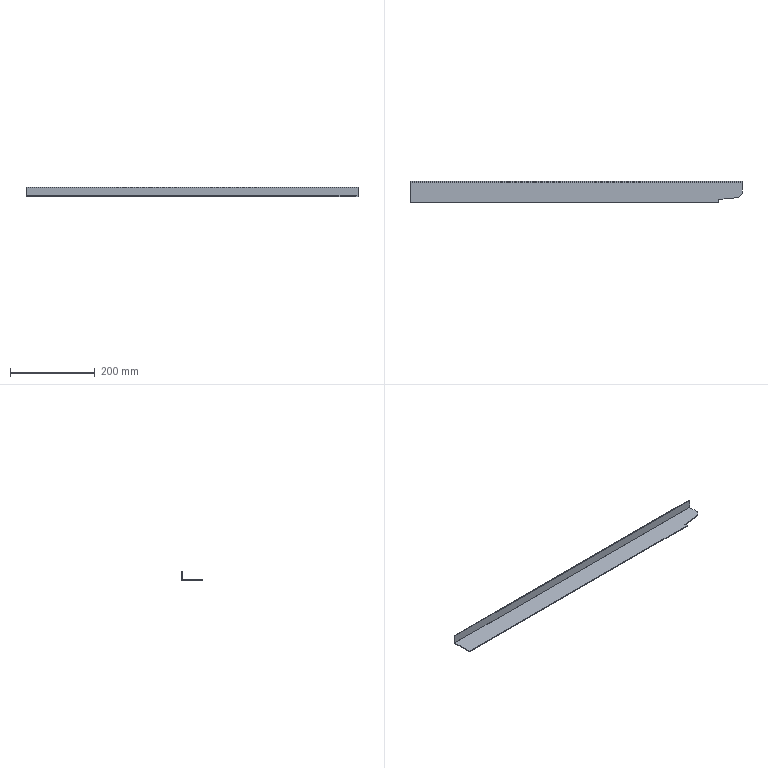Part | SolidWorks | 1 solid | 18 faces | box 783.5 x 50 x 22 mm | volume 107737 mm3 | plane 16 | cylinder 2 | commonest cylinder face diameters 0.2 x1 4.2 x1
STEP:
#1=CARTESIAN_POINT('',(335.25,-25.,-2.));
#2=VERTEX_POINT('',#1);
#3=CARTESIAN_POINT('',(335.25,-17.499,-2.));
#4=VERTEX_POINT('',#3);
#5=CARTESIAN_POINT('',(335.25,0.,-2.));
#6=DIRECTION('',(0.,1.,0.));
#7=VECTOR('',#6,1000.);
#8=LINE('',#5,#7);
#9=EDGE_CURVE('',#2,#4,#8,.T.);
#10=ORIENTED_EDGE('',*,*,#9,.F.);
#11=CARTESIAN_POINT('',(-391.75,-25.,-2.));
#12=VERTEX_POINT('',#11);
#13=CARTESIAN_POINT('',(391.75,-25.,-2.));
#14=DIRECTION('',(1.,0.,0.));
#15=VECTOR('',#14,1000.);
#16=LINE('',#13,#15);
#17=EDGE_CURVE('',#12,#2,#16,.T.);
#18=ORIENTED_EDGE('',*,*,#17,.F.);
#19=CARTESIAN_POINT('',(-391.75,22.9,-2.));
#20=VERTEX_POINT('',#19);
#21=CARTESIAN_POINT('',(-391.75,-25.,-2.));
#22=DIRECTION('',(0.,-1.,0.));
#23=VECTOR('',#22,1000.);
#24=LINE('',#21,#23);
#25=EDGE_CURVE('',#20,#12,#24,.T.);
#26=ORIENTED_EDGE('',*,*,#25,.F.);
#27=CARTESIAN_POINT('',(391.75,22.9,-2.));
#28=VERTEX_POINT('',#27);
#29=CARTESIAN_POINT('',(-391.75,22.9,-2.));
#30=DIRECTION('',(1.,0.,0.));
#31=VECTOR('',#30,1000.);
#32=LINE('',#29,#31);
#33=EDGE_CURVE('',#20,#28,#32,.T.);
#34=ORIENTED_EDGE('',*,*,#33,.T.);
#35=CARTESIAN_POINT('',(391.75,-3.027,-2.));
#36=VERTEX_POINT('',#35);
#37=CARTESIAN_POINT('',(391.75,-25.,-2.));
#38=DIRECTION('',(0.,1.,0.));
#39=VECTOR('',#38,1000.);
#40=LINE('',#37,#39);
#41=EDGE_CURVE('',#36,#28,#40,.T.);
#42=ORIENTED_EDGE('',*,*,#41,.F.);
#43=CARTESIAN_POINT('',(382.795,-12.972,-2.));
#44=VERTEX_POINT('',#43);
#45=CARTESIAN_POINT('',(382.795,-12.972,-2.));
#46=DIRECTION('',(0.6691,0.7431,0.));
#47=VECTOR('',#46,1000.);
#48=LINE('',#45,#47);
#49=EDGE_CURVE('',#44,#36,#48,.T.);
#50=ORIENTED_EDGE('',*,*,#49,.F.);
#51=CARTESIAN_POINT('',(339.727,-17.499,-2.));
#52=VERTEX_POINT('',#51);
#53=CARTESIAN_POINT('',(339.727,-17.499,-2.));
#54=DIRECTION('',(0.9945,0.1045,0.));
#55=VECTOR('',#54,1000.);
#56=LINE('',#53,#55);
#57=EDGE_CURVE('',#52,#44,#56,.T.);
#58=ORIENTED_EDGE('',*,*,#57,.F.);
#59=CARTESIAN_POINT('',(0.,-17.499,-2.));
#60=DIRECTION('',(1.,0.,0.));
#61=VECTOR('',#60,1000.);
#62=LINE('',#59,#61);
#63=EDGE_CURVE('',#4,#52,#62,.T.);
#64=ORIENTED_EDGE('',*,*,#63,.F.);
#65=EDGE_LOOP('',(#10,#18,#26,#34,#42,#50,#58,#64));
#66=FACE_OUTER_BOUND('',#65,.T.);
#67=CARTESIAN_POINT('',(0.,0.,-2.));
#68=DIRECTION('',(0.,0.,1.));
#69=DIRECTION('',(1.,0.,0.));
#70=AXIS2_PLACEMENT_3D('',#67,#68,#69);
#71=PLANE('',#70);
#72=ADVANCED_FACE('',(#66),#71,.F.);
#73=CARTESIAN_POINT('',(-391.75,-25.,0.));
#74=VERTEX_POINT('',#73);
#75=CARTESIAN_POINT('',(335.25,-25.,0.));
#76=VERTEX_POINT('',#75);
#77=CARTESIAN_POINT('',(391.75,-25.,0.));
#78=DIRECTION('',(1.,0.,0.));
#79=VECTOR('',#78,1000.);
#80=LINE('',#77,#79);
#81=EDGE_CURVE('',#74,#76,#80,.T.);
#82=ORIENTED_EDGE('',*,*,#81,.T.);
#83=CARTESIAN_POINT('',(335.25,-17.499,0.));
#84=VERTEX_POINT('',#83);
#85=CARTESIAN_POINT('',(335.25,-25.,0.));
#86=DIRECTION('',(0.,1.,0.));
#87=VECTOR('',#86,1000.);
#88=LINE('',#85,#87);
#89=EDGE_CURVE('',#76,#84,#88,.T.);
#90=ORIENTED_EDGE('',*,*,#89,.T.);
#91=CARTESIAN_POINT('',(339.727,-17.499,0.));
#92=VERTEX_POINT('',#91);
#93=CARTESIAN_POINT('',(335.25,-17.499,0.));
#94=DIRECTION('',(1.,0.,0.));
#95=VECTOR('',#94,1000.);
#96=LINE('',#93,#95);
#97=EDGE_CURVE('',#84,#92,#96,.T.);
#98=ORIENTED_EDGE('',*,*,#97,.T.);
#99=CARTESIAN_POINT('',(382.795,-12.972,0.));
#100=VERTEX_POINT('',#99);
#101=CARTESIAN_POINT('',(339.727,-17.499,0.));
#102=DIRECTION('',(0.9945,0.1045,0.));
#103=VECTOR('',#102,1000.);
#104=LINE('',#101,#103);
#105=EDGE_CURVE('',#92,#100,#104,.T.);
#106=ORIENTED_EDGE('',*,*,#105,.T.);
#107=CARTESIAN_POINT('',(391.75,-3.027,0.));
#108=VERTEX_POINT('',#107);
#109=CARTESIAN_POINT('',(382.795,-12.972,0.));
#110=DIRECTION('',(0.6691,0.7431,0.));
#111=VECTOR('',#110,1000.);
#112=LINE('',#109,#111);
#113=EDGE_CURVE('',#100,#108,#112,.T.);
#114=ORIENTED_EDGE('',*,*,#113,.T.);
#115=CARTESIAN_POINT('',(391.75,22.9,0.));
#116=VERTEX_POINT('',#115);
#117=CARTESIAN_POINT('',(391.75,-25.,0.));
#118=DIRECTION('',(0.,1.,0.));
#119=VECTOR('',#118,1000.);
#120=LINE('',#117,#119);
#121=EDGE_CURVE('',#108,#116,#120,.T.);
#122=ORIENTED_EDGE('',*,*,#121,.T.);
#123=CARTESIAN_POINT('',(-391.75,22.9,0.));
#124=VERTEX_POINT('',#123);
#125=CARTESIAN_POINT('',(-391.75,22.9,0.));
#126=DIRECTION('',(1.,0.,0.));
#127=VECTOR('',#126,1000.);
#128=LINE('',#125,#127);
#129=EDGE_CURVE('',#124,#116,#128,.T.);
#130=ORIENTED_EDGE('',*,*,#129,.F.);
#131=CARTESIAN_POINT('',(-391.75,-25.,0.));
#132=DIRECTION('',(0.,-1.,0.));
#133=VECTOR('',#132,1000.);
#134=LINE('',#131,#133);
#135=EDGE_CURVE('',#124,#74,#134,.T.);
#136=ORIENTED_EDGE('',*,*,#135,.T.);
#137=EDGE_LOOP('',(#82,#90,#98,#106,#114,#122,#130,#136));
#138=FACE_OUTER_BOUND('',#137,.T.);
#139=CARTESIAN_POINT('',(0.,0.,0.));
#140=DIRECTION('',(0.,0.,1.));
#141=DIRECTION('',(1.,0.,0.));
#142=AXIS2_PLACEMENT_3D('',#139,#140,#141);
#143=PLANE('',#142);
#144=ADVANCED_FACE('',(#138),#143,.T.);
#145=ORIENTED_EDGE('',*,*,#121,.F.);
#146=CARTESIAN_POINT('',(391.75,-3.027,0.));
#147=DIRECTION('',(0.,0.,-1.));
#148=VECTOR('',#147,1000.);
#149=LINE('',#146,#148);
#150=EDGE_CURVE('',#108,#36,#149,.T.);
#151=ORIENTED_EDGE('',*,*,#150,.T.);
#152=ORIENTED_EDGE('',*,*,#41,.T.);
#153=CARTESIAN_POINT('',(391.75,22.9,0.));
#154=DIRECTION('',(0.,0.,-1.));
#155=VECTOR('',#154,1000.);
#156=LINE('',#153,#155);
#157=EDGE_CURVE('',#116,#28,#156,.T.);
#158=ORIENTED_EDGE('',*,*,#157,.F.);
#159=EDGE_LOOP('',(#145,#151,#152,#158));
#160=FACE_OUTER_BOUND('',#159,.T.);
#161=CARTESIAN_POINT('',(391.75,-25.,-2.));
#162=DIRECTION('',(1.,0.,0.));
#163=DIRECTION('',(0.,0.,-1.));
#164=AXIS2_PLACEMENT_3D('',#161,#162,#163);
#165=PLANE('',#164);
#166=ADVANCED_FACE('',(#160),#165,.T.);
#167=ORIENTED_EDGE('',*,*,#17,.T.);
#168=CARTESIAN_POINT('',(335.25,-25.,0.));
#169=DIRECTION('',(0.,0.,-1.));
#170=VECTOR('',#169,1000.);
#171=LINE('',#168,#170);
#172=EDGE_CURVE('',#76,#2,#171,.T.);
#173=ORIENTED_EDGE('',*,*,#172,.F.);
#174=ORIENTED_EDGE('',*,*,#81,.F.);
#175=CARTESIAN_POINT('',(-391.75,-25.,-2.));
#176=DIRECTION('',(0.,0.,1.));
#177=VECTOR('',#176,1000.);
#178=LINE('',#175,#177);
#179=EDGE_CURVE('',#12,#74,#178,.T.);
#180=ORIENTED_EDGE('',*,*,#179,.F.);
#181=EDGE_LOOP('',(#167,#173,#174,#180));
#182=FACE_OUTER_BOUND('',#181,.T.);
#183=CARTESIAN_POINT('',(391.75,-25.,-2.));
#184=DIRECTION('',(0.,-1.,0.));
#185=DIRECTION('',(1.,0.,0.));
#186=AXIS2_PLACEMENT_3D('',#183,#184,#185);
#187=PLANE('',#186);
#188=ADVANCED_FACE('',(#182),#187,.T.);
#189=ORIENTED_EDGE('',*,*,#135,.F.);
#190=CARTESIAN_POINT('',(-391.75,22.9,0.));
#191=DIRECTION('',(0.,0.,-1.));
#192=VECTOR('',#191,1000.);
#193=LINE('',#190,#192);
#194=EDGE_CURVE('',#124,#20,#193,.T.);
#195=ORIENTED_EDGE('',*,*,#194,.T.);
#196=ORIENTED_EDGE('',*,*,#25,.T.);
#197=ORIENTED_EDGE('',*,*,#179,.T.);
#198=EDGE_LOOP('',(#189,#195,#196,#197));
#199=FACE_OUTER_BOUND('',#198,.T.);
#200=CARTESIAN_POINT('',(-391.75,-25.,-2.));
#201=DIRECTION('',(-1.,0.,0.));
#202=DIRECTION('',(0.,0.,1.));
#203=AXIS2_PLACEMENT_3D('',#200,#201,#202);
#204=PLANE('',#203);
#205=ADVANCED_FACE('',(#199),#204,.T.);
#206=CARTESIAN_POINT('',(391.75,23.,0.1));
#207=VERTEX_POINT('',#206);
#208=CARTESIAN_POINT('',(391.75,25.,0.1));
#209=VERTEX_POINT('',#208);
#210=CARTESIAN_POINT('',(391.75,25.,0.1));
#211=DIRECTION('',(0.,1.,0.));
#212=VECTOR('',#211,1000.);
#213=LINE('',#210,#212);
#214=EDGE_CURVE('',#207,#209,#213,.T.);
#215=ORIENTED_EDGE('',*,*,#214,.F.);
#216=CARTESIAN_POINT('',(391.75,22.9,0.1));
#217=DIRECTION('',(1.,0.,0.));
#218=DIRECTION('',(0.,0.,1.));
#219=AXIS2_PLACEMENT_3D('',#216,#217,#218);
#220=CIRCLE('',#219,0.1);
#221=EDGE_CURVE('',#116,#207,#220,.T.);
#222=ORIENTED_EDGE('',*,*,#221,.F.);
#223=ORIENTED_EDGE('',*,*,#157,.T.);
#224=CARTESIAN_POINT('',(391.75,22.9,0.1));
#225=DIRECTION('',(1.,0.,0.));
#226=DIRECTION('',(0.,0.,1.));
#227=AXIS2_PLACEMENT_3D('',#224,#225,#226);
#228=CIRCLE('',#227,2.1);
#229=EDGE_CURVE('',#28,#209,#228,.T.);
#230=ORIENTED_EDGE('',*,*,#229,.T.);
#231=EDGE_LOOP('',(#215,#222,#223,#230));
#232=FACE_OUTER_BOUND('',#231,.T.);
#233=CARTESIAN_POINT('',(391.75,22.9,0.1));
#234=DIRECTION('',(1.,0.,0.));
#235=DIRECTION('',(0.,0.,-1.));
#236=AXIS2_PLACEMENT_3D('',#233,#234,#235);
#237=PLANE('',#236);
#238=ADVANCED_FACE('',(#232),#237,.T.);
#239=CARTESIAN_POINT('',(-391.75,23.,0.1));
#240=VERTEX_POINT('',#239);
#241=CARTESIAN_POINT('',(-391.75,22.9,0.1));
#242=DIRECTION('',(-1.,0.,0.));
#243=DIRECTION('',(0.,0.,1.));
#244=AXIS2_PLACEMENT_3D('',#241,#242,#243);
#245=CIRCLE('',#244,0.1);
#246=EDGE_CURVE('',#240,#124,#245,.T.);
#247=ORIENTED_EDGE('',*,*,#246,.F.);
#248=CARTESIAN_POINT('',(-391.75,25.,0.1));
#249=VERTEX_POINT('',#248);
#250=CARTESIAN_POINT('',(-391.75,23.,0.1));
#251=DIRECTION('',(0.,1.,0.));
#252=VECTOR('',#251,1000.);
#253=LINE('',#250,#252);
#254=EDGE_CURVE('',#240,#249,#253,.T.);
#255=ORIENTED_EDGE('',*,*,#254,.T.);
#256=CARTESIAN_POINT('',(-391.75,22.9,0.1));
#257=DIRECTION('',(-1.,0.,0.));
#258=DIRECTION('',(0.,0.,1.));
#259=AXIS2_PLACEMENT_3D('',#256,#257,#258);
#260=CIRCLE('',#259,2.1);
#261=EDGE_CURVE('',#249,#20,#260,.T.);
#262=ORIENTED_EDGE('',*,*,#261,.T.);
#263=ORIENTED_EDGE('',*,*,#194,.F.);
#264=EDGE_LOOP('',(#247,#255,#262,#263));
#265=FACE_OUTER_BOUND('',#264,.T.);
#266=CARTESIAN_POINT('',(-391.75,22.9,0.1));
#267=DIRECTION('',(1.,0.,0.));
#268=DIRECTION('',(0.,0.,-1.));
#269=AXIS2_PLACEMENT_3D('',#266,#267,#268);
#270=PLANE('',#269);
#271=ADVANCED_FACE('',(#265),#270,.F.);
#272=ORIENTED_EDGE('',*,*,#33,.F.);
#273=ORIENTED_EDGE('',*,*,#261,.F.);
#274=CARTESIAN_POINT('',(0.,25.,0.1));
#275=DIRECTION('',(-1.,0.,0.));
#276=VECTOR('',#275,1000.);
#277=LINE('',#274,#276);
#278=EDGE_CURVE('',#209,#249,#277,.T.);
#279=ORIENTED_EDGE('',*,*,#278,.F.);
#280=ORIENTED_EDGE('',*,*,#229,.F.);
#281=EDGE_LOOP('',(#272,#273,#279,#280));
#282=FACE_OUTER_BOUND('',#281,.T.);
#283=CARTESIAN_POINT('',(-391.75,22.9,0.1));
#284=DIRECTION('',(-1.,0.,0.));
#285=DIRECTION('',(0.,1.,0.));
#286=AXIS2_PLACEMENT_3D('',#283,#284,#285);
#287=CYLINDRICAL_SURFACE('',#286,2.1);
#288=ADVANCED_FACE('',(#282),#287,.T.);
#289=ORIENTED_EDGE('',*,*,#129,.T.);
#290=ORIENTED_EDGE('',*,*,#221,.T.);
#291=CARTESIAN_POINT('',(391.75,23.,0.1));
#292=DIRECTION('',(-1.,0.,0.));
#293=VECTOR('',#292,1000.);
#294=LINE('',#291,#293);
#295=EDGE_CURVE('',#207,#240,#294,.T.);
#296=ORIENTED_EDGE('',*,*,#295,.T.);
#297=ORIENTED_EDGE('',*,*,#246,.T.);
#298=EDGE_LOOP('',(#289,#290,#296,#297));
#299=FACE_OUTER_BOUND('',#298,.T.);
#300=CARTESIAN_POINT('',(-391.75,22.9,0.1));
#301=DIRECTION('',(-1.,0.,0.));
#302=DIRECTION('',(0.,1.,0.));
#303=AXIS2_PLACEMENT_3D('',#300,#301,#302);
#304=CYLINDRICAL_SURFACE('',#303,0.1);
#305=ADVANCED_FACE('',(#299),#304,.F.);
#306=CARTESIAN_POINT('',(-391.75,25.,20.));
#307=VERTEX_POINT('',#306);
#308=CARTESIAN_POINT('',(-391.75,25.,0.));
#309=DIRECTION('',(0.,0.,-1.));
#310=VECTOR('',#309,1000.);
#311=LINE('',#308,#310);
#312=EDGE_CURVE('',#307,#249,#311,.T.);
#313=ORIENTED_EDGE('',*,*,#312,.T.);
#314=ORIENTED_EDGE('',*,*,#254,.F.);
#315=CARTESIAN_POINT('',(-391.75,23.,20.));
#316=VERTEX_POINT('',#315);
#317=CARTESIAN_POINT('',(-391.75,23.,0.));
#318=DIRECTION('',(0.,0.,-1.));
#319=VECTOR('',#318,1000.);
#320=LINE('',#317,#319);
#321=EDGE_CURVE('',#316,#240,#320,.T.);
#322=ORIENTED_EDGE('',*,*,#321,.F.);
#323=CARTESIAN_POINT('',(-391.75,25.,20.));
#324=DIRECTION('',(0.,-1.,0.));
#325=VECTOR('',#324,1000.);
#326=LINE('',#323,#325);
#327=EDGE_CURVE('',#307,#316,#326,.T.);
#328=ORIENTED_EDGE('',*,*,#327,.F.);
#329=EDGE_LOOP('',(#313,#314,#322,#328));
#330=FACE_OUTER_BOUND('',#329,.T.);
#331=CARTESIAN_POINT('',(-391.75,25.,0.));
#332=DIRECTION('',(-1.,0.,0.));
#333=DIRECTION('',(0.,-1.,0.));
#334=AXIS2_PLACEMENT_3D('',#331,#332,#333);
#335=PLANE('',#334);
#336=ADVANCED_FACE('',(#330),#335,.T.);
#337=CARTESIAN_POINT('',(391.75,23.,20.));
#338=VERTEX_POINT('',#337);
#339=CARTESIAN_POINT('',(391.75,23.,0.));
#340=DIRECTION('',(0.,0.,1.));
#341=VECTOR('',#340,1000.);
#342=LINE('',#339,#341);
#343=EDGE_CURVE('',#207,#338,#342,.T.);
#344=ORIENTED_EDGE('',*,*,#343,.F.);
#345=ORIENTED_EDGE('',*,*,#214,.T.);
#346=CARTESIAN_POINT('',(391.75,25.,20.));
#347=VERTEX_POINT('',#346);
#348=CARTESIAN_POINT('',(391.75,25.,20.));
#349=DIRECTION('',(0.,0.,1.));
#350=VECTOR('',#349,1000.);
#351=LINE('',#348,#350);
#352=EDGE_CURVE('',#209,#347,#351,.T.);
#353=ORIENTED_EDGE('',*,*,#352,.T.);
#354=CARTESIAN_POINT('',(391.75,25.,20.));
#355=DIRECTION('',(0.,-1.,0.));
#356=VECTOR('',#355,1000.);
#357=LINE('',#354,#356);
#358=EDGE_CURVE('',#347,#338,#357,.T.);
#359=ORIENTED_EDGE('',*,*,#358,.T.);
#360=EDGE_LOOP('',(#344,#345,#353,#359));
#361=FACE_OUTER_BOUND('',#360,.T.);
#362=CARTESIAN_POINT('',(391.75,25.,20.));
#363=DIRECTION('',(1.,0.,0.));
#364=DIRECTION('',(0.,1.,0.));
#365=AXIS2_PLACEMENT_3D('',#362,#363,#364);
#366=PLANE('',#365);
#367=ADVANCED_FACE('',(#361),#366,.T.);
#368=ORIENTED_EDGE('',*,*,#352,.F.);
#369=ORIENTED_EDGE('',*,*,#278,.T.);
#370=ORIENTED_EDGE('',*,*,#312,.F.);
#371=CARTESIAN_POINT('',(-391.75,25.,20.));
#372=DIRECTION('',(-1.,0.,0.));
#373=VECTOR('',#372,1000.);
#374=LINE('',#371,#373);
#375=EDGE_CURVE('',#347,#307,#374,.T.);
#376=ORIENTED_EDGE('',*,*,#375,.F.);
#377=EDGE_LOOP('',(#368,#369,#370,#376));
#378=FACE_OUTER_BOUND('',#377,.T.);
#379=CARTESIAN_POINT('',(0.,25.,0.));
#380=DIRECTION('',(0.,1.,0.));
#381=DIRECTION('',(0.,0.,1.));
#382=AXIS2_PLACEMENT_3D('',#379,#380,#381);
#383=PLANE('',#382);
#384=ADVANCED_FACE('',(#378),#383,.T.);
#385=ORIENTED_EDGE('',*,*,#295,.F.);
#386=ORIENTED_EDGE('',*,*,#343,.T.);
#387=CARTESIAN_POINT('',(0.,23.,20.));
#388=DIRECTION('',(-1.,0.,0.));
#389=VECTOR('',#388,1000.);
#390=LINE('',#387,#389);
#391=EDGE_CURVE('',#338,#316,#390,.T.);
#392=ORIENTED_EDGE('',*,*,#391,.T.);
#393=ORIENTED_EDGE('',*,*,#321,.T.);
#394=EDGE_LOOP('',(#385,#386,#392,#393));
#395=FACE_OUTER_BOUND('',#394,.T.);
#396=CARTESIAN_POINT('',(0.,23.,0.));
#397=DIRECTION('',(0.,1.,0.));
#398=DIRECTION('',(0.,0.,1.));
#399=AXIS2_PLACEMENT_3D('',#396,#397,#398);
#400=PLANE('',#399);
#401=ADVANCED_FACE('',(#395),#400,.F.);
#402=ORIENTED_EDGE('',*,*,#391,.F.);
#403=ORIENTED_EDGE('',*,*,#358,.F.);
#404=ORIENTED_EDGE('',*,*,#375,.T.);
#405=ORIENTED_EDGE('',*,*,#327,.T.);
#406=EDGE_LOOP('',(#402,#403,#404,#405));
#407=FACE_OUTER_BOUND('',#406,.T.);
#408=CARTESIAN_POINT('',(-391.75,25.,20.));
#409=DIRECTION('',(0.,0.,1.));
#410=DIRECTION('',(0.,-1.,0.));
#411=AXIS2_PLACEMENT_3D('',#408,#409,#410);
#412=PLANE('',#411);
#413=ADVANCED_FACE('',(#407),#412,.T.);
#414=CARTESIAN_POINT('',(382.795,-12.972,0.));
#415=DIRECTION('',(0.,0.,-1.));
#416=VECTOR('',#415,1000.);
#417=LINE('',#414,#416);
#418=EDGE_CURVE('',#100,#44,#417,.T.);
#419=ORIENTED_EDGE('',*,*,#418,.F.);
#420=ORIENTED_EDGE('',*,*,#105,.F.);
#421=CARTESIAN_POINT('',(339.727,-17.499,0.));
#422=DIRECTION('',(0.,0.,-1.));
#423=VECTOR('',#422,1000.);
#424=LINE('',#421,#423);
#425=EDGE_CURVE('',#92,#52,#424,.T.);
#426=ORIENTED_EDGE('',*,*,#425,.T.);
#427=ORIENTED_EDGE('',*,*,#57,.T.);
#428=EDGE_LOOP('',(#419,#420,#426,#427));
#429=FACE_OUTER_BOUND('',#428,.T.);
#430=CARTESIAN_POINT('',(339.727,-17.499,0.));
#431=DIRECTION('',(0.1045,-0.9945,0.));
#432=DIRECTION('',(0.9945,0.1045,0.));
#433=AXIS2_PLACEMENT_3D('',#430,#431,#432);
#434=PLANE('',#433);
#435=ADVANCED_FACE('',(#429),#434,.T.);
#436=ORIENTED_EDGE('',*,*,#425,.F.);
#437=ORIENTED_EDGE('',*,*,#97,.F.);
#438=CARTESIAN_POINT('',(335.25,-17.499,0.));
#439=DIRECTION('',(0.,0.,-1.));
#440=VECTOR('',#439,1000.);
#441=LINE('',#438,#440);
#442=EDGE_CURVE('',#84,#4,#441,.T.);
#443=ORIENTED_EDGE('',*,*,#442,.T.);
#444=ORIENTED_EDGE('',*,*,#63,.T.);
#445=EDGE_LOOP('',(#436,#437,#443,#444));
#446=FACE_OUTER_BOUND('',#445,.T.);
#447=CARTESIAN_POINT('',(335.25,-17.499,0.));
#448=DIRECTION('',(0.,-1.,0.));
#449=DIRECTION('',(1.,0.,0.));
#450=AXIS2_PLACEMENT_3D('',#447,#448,#449);
#451=PLANE('',#450);
#452=ADVANCED_FACE('',(#446),#451,.T.);
#453=ORIENTED_EDGE('',*,*,#442,.F.);
#454=ORIENTED_EDGE('',*,*,#89,.F.);
#455=ORIENTED_EDGE('',*,*,#172,.T.);
#456=ORIENTED_EDGE('',*,*,#9,.T.);
#457=EDGE_LOOP('',(#453,#454,#455,#456));
#458=FACE_OUTER_BOUND('',#457,.T.);
#459=CARTESIAN_POINT('',(335.25,-25.,0.));
#460=DIRECTION('',(1.,0.,0.));
#461=DIRECTION('',(0.,1.,0.));
#462=AXIS2_PLACEMENT_3D('',#459,#460,#461);
#463=PLANE('',#462);
#464=ADVANCED_FACE('',(#458),#463,.T.);
#465=ORIENTED_EDGE('',*,*,#113,.F.);
#466=ORIENTED_EDGE('',*,*,#418,.T.);
#467=ORIENTED_EDGE('',*,*,#49,.T.);
#468=ORIENTED_EDGE('',*,*,#150,.F.);
#469=EDGE_LOOP('',(#465,#466,#467,#468));
#470=FACE_OUTER_BOUND('',#469,.T.);
#471=CARTESIAN_POINT('',(382.795,-12.972,0.));
#472=DIRECTION('',(0.7431,-0.6691,0.));
#473=DIRECTION('',(0.6691,0.7431,0.));
#474=AXIS2_PLACEMENT_3D('',#471,#472,#473);
#475=PLANE('',#474);
#476=ADVANCED_FACE('',(#470),#475,.T.);
#477=CLOSED_SHELL('',(#72,#144,#166,#188,#205,#238,#271,#288,#305,#336,#367,#384,#401,#413,#435,#452,#464,#476));
#478=MANIFOLD_SOLID_BREP('',#477);
#479=CARTESIAN_POINT('',(0.,0.,0.));
#480=DIRECTION('',(0.,0.,1.));
#481=DIRECTION('',(1.,0.,0.));
#482=AXIS2_PLACEMENT_3D('',#479,#480,#481);
#483=(LENGTH_UNIT()NAMED_UNIT(*)SI_UNIT(.MILLI.,.METRE.));
#484=UNCERTAINTY_MEASURE_WITH_UNIT(LENGTH_MEASURE(0.00001),#483,'','');
#485=(NAMED_UNIT(*)PLANE_ANGLE_UNIT()SI_UNIT($,.RADIAN.));
#486=(NAMED_UNIT(*)SI_UNIT($,.STERADIAN.)SOLID_ANGLE_UNIT());
#487=(GEOMETRIC_REPRESENTATION_CONTEXT(3)GLOBAL_UNCERTAINTY_ASSIGNED_CONTEXT((#484))GLOBAL_UNIT_ASSIGNED_CONTEXT((#483,#485,#486))REPRESENTATION_CONTEXT('',''));
#488=ADVANCED_BREP_SHAPE_REPRESENTATION('',(#478,#482),#487);